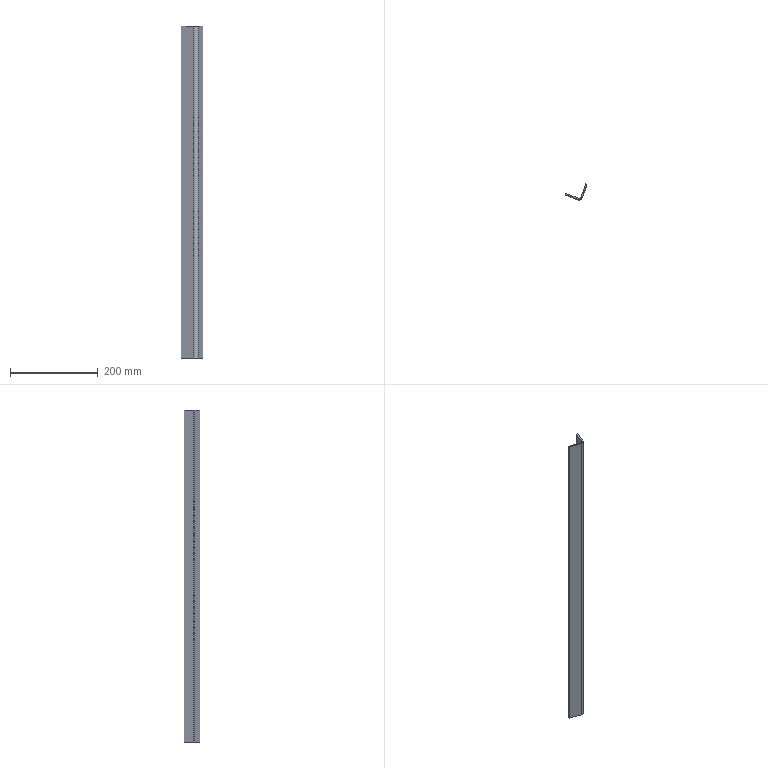Part | SolidWorks | features FlatPattern 1, SMBaseFlange 1, SheetMetal 1 | 1 solid | 14 faces | box 49.987 x 35.42 x 758 mm | volume 164206 mm3 | plane 12 | cylinder 2 | commonest cylinder face diameters 10 x1 16 x1
STEP:
#1=CARTESIAN_POINT('',(299.338,278.733,-758.));
#2=VERTEX_POINT('',#1);
#3=CARTESIAN_POINT('',(296.519,279.759,-758.));
#4=VERTEX_POINT('',#3);
#5=CARTESIAN_POINT('',(299.338,278.733,-758.));
#6=DIRECTION('',(-0.9397,0.342,0.));
#7=VECTOR('',#6,1000.);
#8=LINE('',#5,#7);
#9=EDGE_CURVE('',#2,#4,#8,.T.);
#10=ORIENTED_EDGE('',*,*,#9,.F.);
#11=CARTESIAN_POINT('',(289.085,273.952,-758.));
#12=VERTEX_POINT('',#11);
#13=CARTESIAN_POINT('',(291.821,281.469,-758.));
#14=DIRECTION('',(0.,0.,-1.));
#15=DIRECTION('',(1.,0.,0.));
#16=AXIS2_PLACEMENT_3D('',#13,#14,#15);
#17=CIRCLE('',#16,8.);
#18=EDGE_CURVE('',#2,#12,#17,.T.);
#19=ORIENTED_EDGE('',*,*,#18,.T.);
#20=CARTESIAN_POINT('',(290.111,276.771,-758.));
#21=VERTEX_POINT('',#20);
#22=CARTESIAN_POINT('',(290.111,276.771,-758.));
#23=DIRECTION('',(-0.342,-0.9397,0.));
#24=VECTOR('',#23,1000.);
#25=LINE('',#22,#24);
#26=EDGE_CURVE('',#21,#12,#25,.T.);
#27=ORIENTED_EDGE('',*,*,#26,.F.);
#28=CARTESIAN_POINT('',(291.821,281.469,-758.));
#29=DIRECTION('',(0.,0.,-1.));
#30=DIRECTION('',(1.,0.,0.));
#31=AXIS2_PLACEMENT_3D('',#28,#29,#30);
#32=CIRCLE('',#31,5.);
#33=EDGE_CURVE('',#4,#21,#32,.T.);
#34=ORIENTED_EDGE('',*,*,#33,.F.);
#35=EDGE_LOOP('',(#10,#19,#27,#34));
#36=FACE_OUTER_BOUND('',#35,.T.);
#37=CARTESIAN_POINT('',(299.338,278.733,-758.));
#38=DIRECTION('',(0.,0.,-1.));
#39=DIRECTION('',(-1.,0.,0.));
#40=AXIS2_PLACEMENT_3D('',#37,#38,#39);
#41=PLANE('',#40);
#42=ADVANCED_FACE('',(#36),#41,.T.);
#43=CARTESIAN_POINT('',(309.941,307.863,-758.));
#44=VERTEX_POINT('',#43);
#45=CARTESIAN_POINT('',(309.941,307.863,-758.));
#46=DIRECTION('',(-0.342,-0.9397,0.));
#47=VECTOR('',#46,1000.);
#48=LINE('',#45,#47);
#49=EDGE_CURVE('',#44,#2,#48,.T.);
#50=ORIENTED_EDGE('',*,*,#49,.T.);
#51=ORIENTED_EDGE('',*,*,#9,.T.);
#52=CARTESIAN_POINT('',(307.122,308.889,-758.));
#53=VERTEX_POINT('',#52);
#54=CARTESIAN_POINT('',(307.122,308.889,-758.));
#55=DIRECTION('',(-0.342,-0.9397,0.));
#56=VECTOR('',#55,1000.);
#57=LINE('',#54,#56);
#58=EDGE_CURVE('',#53,#4,#57,.T.);
#59=ORIENTED_EDGE('',*,*,#58,.F.);
#60=CARTESIAN_POINT('',(307.122,308.889,-758.));
#61=DIRECTION('',(0.9397,-0.342,0.));
#62=VECTOR('',#61,1000.);
#63=LINE('',#60,#62);
#64=EDGE_CURVE('',#53,#44,#63,.T.);
#65=ORIENTED_EDGE('',*,*,#64,.T.);
#66=EDGE_LOOP('',(#50,#51,#59,#65));
#67=FACE_OUTER_BOUND('',#66,.T.);
#68=CARTESIAN_POINT('',(290.111,276.771,-758.));
#69=DIRECTION('',(0.,0.,-1.));
#70=DIRECTION('',(-1.,0.,0.));
#71=AXIS2_PLACEMENT_3D('',#68,#69,#70);
#72=PLANE('',#71);
#73=ADVANCED_FACE('',(#67),#72,.T.);
#74=CARTESIAN_POINT('',(289.085,273.952,0.));
#75=VERTEX_POINT('',#74);
#76=CARTESIAN_POINT('',(290.111,276.771,0.));
#77=VERTEX_POINT('',#76);
#78=CARTESIAN_POINT('',(289.085,273.952,0.));
#79=DIRECTION('',(0.342,0.9397,0.));
#80=VECTOR('',#79,1000.);
#81=LINE('',#78,#80);
#82=EDGE_CURVE('',#75,#77,#81,.T.);
#83=ORIENTED_EDGE('',*,*,#82,.F.);
#84=CARTESIAN_POINT('',(299.338,278.733,0.));
#85=VERTEX_POINT('',#84);
#86=CARTESIAN_POINT('',(291.821,281.469,0.));
#87=DIRECTION('',(0.,0.,-1.));
#88=DIRECTION('',(1.,0.,0.));
#89=AXIS2_PLACEMENT_3D('',#86,#87,#88);
#90=CIRCLE('',#89,8.);
#91=EDGE_CURVE('',#85,#75,#90,.T.);
#92=ORIENTED_EDGE('',*,*,#91,.F.);
#93=CARTESIAN_POINT('',(296.519,279.759,0.));
#94=VERTEX_POINT('',#93);
#95=CARTESIAN_POINT('',(296.519,279.759,0.));
#96=DIRECTION('',(0.9397,-0.342,0.));
#97=VECTOR('',#96,1000.);
#98=LINE('',#95,#97);
#99=EDGE_CURVE('',#94,#85,#98,.T.);
#100=ORIENTED_EDGE('',*,*,#99,.F.);
#101=CARTESIAN_POINT('',(291.821,281.469,0.));
#102=DIRECTION('',(0.,0.,-1.));
#103=DIRECTION('',(1.,0.,0.));
#104=AXIS2_PLACEMENT_3D('',#101,#102,#103);
#105=CIRCLE('',#104,5.);
#106=EDGE_CURVE('',#94,#77,#105,.T.);
#107=ORIENTED_EDGE('',*,*,#106,.T.);
#108=EDGE_LOOP('',(#83,#92,#100,#107));
#109=FACE_OUTER_BOUND('',#108,.T.);
#110=CARTESIAN_POINT('',(289.085,273.952,0.));
#111=DIRECTION('',(0.,0.,1.));
#112=DIRECTION('',(1.,0.,0.));
#113=AXIS2_PLACEMENT_3D('',#110,#111,#112);
#114=PLANE('',#113);
#115=ADVANCED_FACE('',(#109),#114,.T.);
#116=CARTESIAN_POINT('',(259.954,284.554,0.));
#117=VERTEX_POINT('',#116);
#118=CARTESIAN_POINT('',(296.602,271.215,0.));
#119=DIRECTION('',(-0.9397,0.342,0.));
#120=VECTOR('',#119,1000.);
#121=LINE('',#118,#120);
#122=EDGE_CURVE('',#75,#117,#121,.T.);
#123=ORIENTED_EDGE('',*,*,#122,.F.);
#124=ORIENTED_EDGE('',*,*,#82,.T.);
#125=CARTESIAN_POINT('',(260.98,287.373,0.));
#126=VERTEX_POINT('',#125);
#127=CARTESIAN_POINT('',(297.628,274.034,0.));
#128=DIRECTION('',(-0.9397,0.342,0.));
#129=VECTOR('',#128,1000.);
#130=LINE('',#127,#129);
#131=EDGE_CURVE('',#77,#126,#130,.T.);
#132=ORIENTED_EDGE('',*,*,#131,.T.);
#133=CARTESIAN_POINT('',(259.954,284.554,0.));
#134=DIRECTION('',(0.342,0.9397,0.));
#135=VECTOR('',#134,1000.);
#136=LINE('',#133,#135);
#137=EDGE_CURVE('',#117,#126,#136,.T.);
#138=ORIENTED_EDGE('',*,*,#137,.F.);
#139=EDGE_LOOP('',(#123,#124,#132,#138));
#140=FACE_OUTER_BOUND('',#139,.T.);
#141=CARTESIAN_POINT('',(296.519,279.759,0.));
#142=DIRECTION('',(0.,0.,1.));
#143=DIRECTION('',(1.,0.,0.));
#144=AXIS2_PLACEMENT_3D('',#141,#142,#143);
#145=PLANE('',#144);
#146=ADVANCED_FACE('',(#140),#145,.T.);
#147=ORIENTED_EDGE('',*,*,#131,.F.);
#148=CARTESIAN_POINT('',(290.111,276.771,-758.));
#149=DIRECTION('',(0.,0.,1.));
#150=VECTOR('',#149,1000.);
#151=LINE('',#148,#150);
#152=EDGE_CURVE('',#21,#77,#151,.T.);
#153=ORIENTED_EDGE('',*,*,#152,.F.);
#154=CARTESIAN_POINT('',(260.98,287.373,-758.));
#155=VERTEX_POINT('',#154);
#156=CARTESIAN_POINT('',(297.628,274.034,-758.));
#157=DIRECTION('',(-0.9397,0.342,0.));
#158=VECTOR('',#157,1000.);
#159=LINE('',#156,#158);
#160=EDGE_CURVE('',#21,#155,#159,.T.);
#161=ORIENTED_EDGE('',*,*,#160,.T.);
#162=CARTESIAN_POINT('',(260.98,287.373,-758.));
#163=DIRECTION('',(0.,0.,1.));
#164=VECTOR('',#163,1000.);
#165=LINE('',#162,#164);
#166=EDGE_CURVE('',#155,#126,#165,.T.);
#167=ORIENTED_EDGE('',*,*,#166,.T.);
#168=EDGE_LOOP('',(#147,#153,#161,#167));
#169=FACE_OUTER_BOUND('',#168,.T.);
#170=CARTESIAN_POINT('',(297.628,274.034,-758.));
#171=DIRECTION('',(0.342,0.9397,0.));
#172=DIRECTION('',(-0.9397,0.342,0.));
#173=AXIS2_PLACEMENT_3D('',#170,#171,#172);
#174=PLANE('',#173);
#175=ADVANCED_FACE('',(#169),#174,.T.);
#176=ORIENTED_EDGE('',*,*,#106,.F.);
#177=CARTESIAN_POINT('',(296.519,279.759,-758.));
#178=DIRECTION('',(0.,0.,1.));
#179=VECTOR('',#178,1000.);
#180=LINE('',#177,#179);
#181=EDGE_CURVE('',#4,#94,#180,.T.);
#182=ORIENTED_EDGE('',*,*,#181,.F.);
#183=ORIENTED_EDGE('',*,*,#33,.T.);
#184=ORIENTED_EDGE('',*,*,#152,.T.);
#185=EDGE_LOOP('',(#176,#182,#183,#184));
#186=FACE_OUTER_BOUND('',#185,.T.);
#187=CARTESIAN_POINT('',(291.821,281.469,-758.));
#188=DIRECTION('',(0.,0.,1.));
#189=DIRECTION('',(1.,0.,0.));
#190=AXIS2_PLACEMENT_3D('',#187,#188,#189);
#191=CYLINDRICAL_SURFACE('',#190,5.);
#192=ADVANCED_FACE('',(#186),#191,.F.);
#193=CARTESIAN_POINT('',(307.122,308.889,0.));
#194=VERTEX_POINT('',#193);
#195=CARTESIAN_POINT('',(307.122,308.889,0.));
#196=DIRECTION('',(-0.342,-0.9397,0.));
#197=VECTOR('',#196,1000.);
#198=LINE('',#195,#197);
#199=EDGE_CURVE('',#194,#94,#198,.T.);
#200=ORIENTED_EDGE('',*,*,#199,.F.);
#201=CARTESIAN_POINT('',(307.122,308.889,-758.));
#202=DIRECTION('',(0.,0.,1.));
#203=VECTOR('',#202,1000.);
#204=LINE('',#201,#203);
#205=EDGE_CURVE('',#53,#194,#204,.T.);
#206=ORIENTED_EDGE('',*,*,#205,.F.);
#207=ORIENTED_EDGE('',*,*,#58,.T.);
#208=ORIENTED_EDGE('',*,*,#181,.T.);
#209=EDGE_LOOP('',(#200,#206,#207,#208));
#210=FACE_OUTER_BOUND('',#209,.T.);
#211=CARTESIAN_POINT('',(307.122,308.889,-758.));
#212=DIRECTION('',(-0.9397,0.342,0.));
#213=DIRECTION('',(-0.342,-0.9397,0.));
#214=AXIS2_PLACEMENT_3D('',#211,#212,#213);
#215=PLANE('',#214);
#216=ADVANCED_FACE('',(#210),#215,.T.);
#217=CARTESIAN_POINT('',(309.941,307.863,0.));
#218=VERTEX_POINT('',#217);
#219=CARTESIAN_POINT('',(307.122,308.889,0.));
#220=DIRECTION('',(0.9397,-0.342,0.));
#221=VECTOR('',#220,1000.);
#222=LINE('',#219,#221);
#223=EDGE_CURVE('',#194,#218,#222,.T.);
#224=ORIENTED_EDGE('',*,*,#223,.T.);
#225=CARTESIAN_POINT('',(309.941,307.863,-758.));
#226=DIRECTION('',(0.,0.,1.));
#227=VECTOR('',#226,1000.);
#228=LINE('',#225,#227);
#229=EDGE_CURVE('',#44,#218,#228,.T.);
#230=ORIENTED_EDGE('',*,*,#229,.F.);
#231=ORIENTED_EDGE('',*,*,#64,.F.);
#232=ORIENTED_EDGE('',*,*,#205,.T.);
#233=EDGE_LOOP('',(#224,#230,#231,#232));
#234=FACE_OUTER_BOUND('',#233,.T.);
#235=CARTESIAN_POINT('',(307.122,308.889,-758.));
#236=DIRECTION('',(-0.342,-0.9397,0.));
#237=DIRECTION('',(0.9397,-0.342,0.));
#238=AXIS2_PLACEMENT_3D('',#235,#236,#237);
#239=PLANE('',#238);
#240=ADVANCED_FACE('',(#234),#239,.F.);
#241=CARTESIAN_POINT('',(309.941,307.863,0.));
#242=DIRECTION('',(-0.342,-0.9397,0.));
#243=VECTOR('',#242,1000.);
#244=LINE('',#241,#243);
#245=EDGE_CURVE('',#218,#85,#244,.T.);
#246=ORIENTED_EDGE('',*,*,#245,.T.);
#247=CARTESIAN_POINT('',(299.338,278.733,-758.));
#248=DIRECTION('',(0.,0.,1.));
#249=VECTOR('',#248,1000.);
#250=LINE('',#247,#249);
#251=EDGE_CURVE('',#2,#85,#250,.T.);
#252=ORIENTED_EDGE('',*,*,#251,.F.);
#253=ORIENTED_EDGE('',*,*,#49,.F.);
#254=ORIENTED_EDGE('',*,*,#229,.T.);
#255=EDGE_LOOP('',(#246,#252,#253,#254));
#256=FACE_OUTER_BOUND('',#255,.T.);
#257=CARTESIAN_POINT('',(309.941,307.863,-758.));
#258=DIRECTION('',(-0.9397,0.342,0.));
#259=DIRECTION('',(-0.342,-0.9397,0.));
#260=AXIS2_PLACEMENT_3D('',#257,#258,#259);
#261=PLANE('',#260);
#262=ADVANCED_FACE('',(#256),#261,.F.);
#263=ORIENTED_EDGE('',*,*,#91,.T.);
#264=CARTESIAN_POINT('',(289.085,273.952,-758.));
#265=DIRECTION('',(0.,0.,1.));
#266=VECTOR('',#265,1000.);
#267=LINE('',#264,#266);
#268=EDGE_CURVE('',#12,#75,#267,.T.);
#269=ORIENTED_EDGE('',*,*,#268,.F.);
#270=ORIENTED_EDGE('',*,*,#18,.F.);
#271=ORIENTED_EDGE('',*,*,#251,.T.);
#272=EDGE_LOOP('',(#263,#269,#270,#271));
#273=FACE_OUTER_BOUND('',#272,.T.);
#274=CARTESIAN_POINT('',(291.821,281.469,-758.));
#275=DIRECTION('',(0.,0.,1.));
#276=DIRECTION('',(1.,0.,0.));
#277=AXIS2_PLACEMENT_3D('',#274,#275,#276);
#278=CYLINDRICAL_SURFACE('',#277,8.);
#279=ADVANCED_FACE('',(#273),#278,.T.);
#280=ORIENTED_EDGE('',*,*,#122,.T.);
#281=CARTESIAN_POINT('',(259.954,284.554,-758.));
#282=VERTEX_POINT('',#281);
#283=CARTESIAN_POINT('',(259.954,284.554,-758.));
#284=DIRECTION('',(0.,0.,1.));
#285=VECTOR('',#284,1000.);
#286=LINE('',#283,#285);
#287=EDGE_CURVE('',#282,#117,#286,.T.);
#288=ORIENTED_EDGE('',*,*,#287,.F.);
#289=CARTESIAN_POINT('',(296.602,271.215,-758.));
#290=DIRECTION('',(-0.9397,0.342,0.));
#291=VECTOR('',#290,1000.);
#292=LINE('',#289,#291);
#293=EDGE_CURVE('',#12,#282,#292,.T.);
#294=ORIENTED_EDGE('',*,*,#293,.F.);
#295=ORIENTED_EDGE('',*,*,#268,.T.);
#296=EDGE_LOOP('',(#280,#288,#294,#295));
#297=FACE_OUTER_BOUND('',#296,.T.);
#298=CARTESIAN_POINT('',(296.602,271.215,-758.));
#299=DIRECTION('',(0.342,0.9397,0.));
#300=DIRECTION('',(-0.9397,0.342,0.));
#301=AXIS2_PLACEMENT_3D('',#298,#299,#300);
#302=PLANE('',#301);
#303=ADVANCED_FACE('',(#297),#302,.F.);
#304=ORIENTED_EDGE('',*,*,#137,.T.);
#305=ORIENTED_EDGE('',*,*,#166,.F.);
#306=CARTESIAN_POINT('',(259.954,284.554,-758.));
#307=DIRECTION('',(0.342,0.9397,0.));
#308=VECTOR('',#307,1000.);
#309=LINE('',#306,#308);
#310=EDGE_CURVE('',#282,#155,#309,.T.);
#311=ORIENTED_EDGE('',*,*,#310,.F.);
#312=ORIENTED_EDGE('',*,*,#287,.T.);
#313=EDGE_LOOP('',(#304,#305,#311,#312));
#314=FACE_OUTER_BOUND('',#313,.T.);
#315=CARTESIAN_POINT('',(259.954,284.554,-758.));
#316=DIRECTION('',(0.9397,-0.342,0.));
#317=DIRECTION('',(0.342,0.9397,0.));
#318=AXIS2_PLACEMENT_3D('',#315,#316,#317);
#319=PLANE('',#318);
#320=ADVANCED_FACE('',(#314),#319,.F.);
#321=ORIENTED_EDGE('',*,*,#160,.F.);
#322=ORIENTED_EDGE('',*,*,#26,.T.);
#323=ORIENTED_EDGE('',*,*,#293,.T.);
#324=ORIENTED_EDGE('',*,*,#310,.T.);
#325=EDGE_LOOP('',(#321,#322,#323,#324));
#326=FACE_OUTER_BOUND('',#325,.T.);
#327=CARTESIAN_POINT('',(291.821,281.469,-758.));
#328=DIRECTION('',(0.,0.,1.));
#329=DIRECTION('',(1.,0.,0.));
#330=AXIS2_PLACEMENT_3D('',#327,#328,#329);
#331=PLANE('',#330);
#332=ADVANCED_FACE('',(#326),#331,.F.);
#333=ORIENTED_EDGE('',*,*,#199,.T.);
#334=ORIENTED_EDGE('',*,*,#99,.T.);
#335=ORIENTED_EDGE('',*,*,#245,.F.);
#336=ORIENTED_EDGE('',*,*,#223,.F.);
#337=EDGE_LOOP('',(#333,#334,#335,#336));
#338=FACE_OUTER_BOUND('',#337,.T.);
#339=CARTESIAN_POINT('',(291.821,281.469,0.));
#340=DIRECTION('',(0.,0.,1.));
#341=DIRECTION('',(1.,0.,0.));
#342=AXIS2_PLACEMENT_3D('',#339,#340,#341);
#343=PLANE('',#342);
#344=ADVANCED_FACE('',(#338),#343,.T.);
#345=CLOSED_SHELL('',(#42,#73,#115,#146,#175,#192,#216,#240,#262,#279,#303,#320,#332,#344));
#346=MANIFOLD_SOLID_BREP('',#345);
#347=CARTESIAN_POINT('',(0.,0.,0.));
#348=DIRECTION('',(0.,0.,1.));
#349=DIRECTION('',(1.,0.,0.));
#350=AXIS2_PLACEMENT_3D('',#347,#348,#349);
#351=(LENGTH_UNIT()NAMED_UNIT(*)SI_UNIT(.MILLI.,.METRE.));
#352=UNCERTAINTY_MEASURE_WITH_UNIT(LENGTH_MEASURE(0.00001),#351,'','');
#353=(NAMED_UNIT(*)PLANE_ANGLE_UNIT()SI_UNIT($,.RADIAN.));
#354=(NAMED_UNIT(*)SI_UNIT($,.STERADIAN.)SOLID_ANGLE_UNIT());
#355=(GEOMETRIC_REPRESENTATION_CONTEXT(3)GLOBAL_UNCERTAINTY_ASSIGNED_CONTEXT((#352))GLOBAL_UNIT_ASSIGNED_CONTEXT((#351,#353,#354))REPRESENTATION_CONTEXT('',''));
#356=ADVANCED_BREP_SHAPE_REPRESENTATION('',(#346,#350),#355);